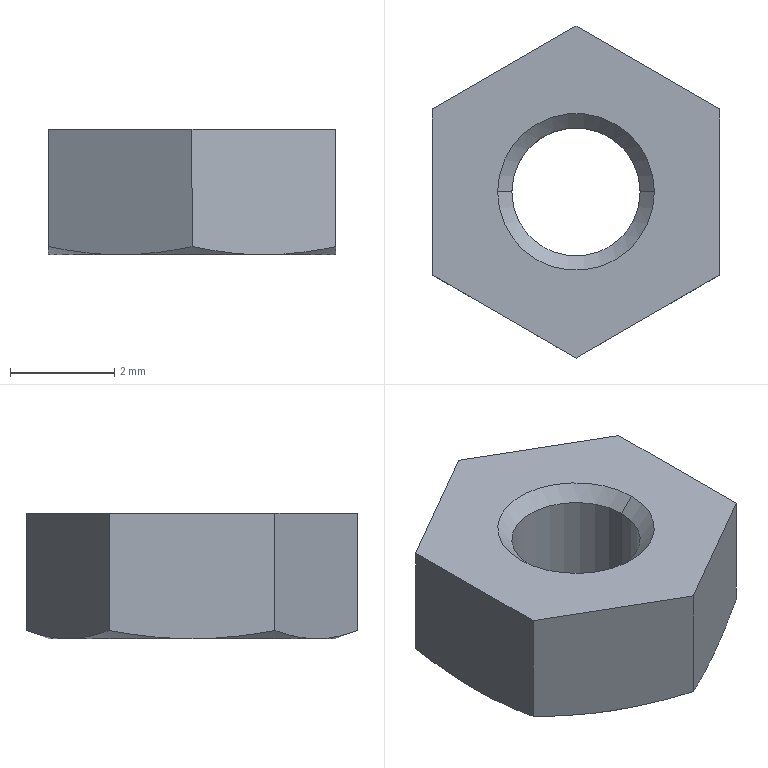Part | SolidWorks | features BaseBody 1 | 1 solid | 20 faces | box 5.5 x 6.351 x 2.4 mm | volume 50.752 mm3 | cone 10 | plane 8 | cylinder 2 | commonest cylinder face diameters 2.459 x2
STEP:
#1=CARTESIAN_POINT('',(-1.23,0.,2.13));
#2=VERTEX_POINT('',#1);
#3=CARTESIAN_POINT('',(1.23,0.,2.13));
#4=VERTEX_POINT('',#3);
#5=CARTESIAN_POINT('',(0.,0.,2.13));
#6=DIRECTION('',(0.,0.,1.));
#7=DIRECTION('',(1.,0.,0.));
#8=AXIS2_PLACEMENT_3D('',#5,#6,#7);
#9=CIRCLE('',#8,1.23);
#10=EDGE_CURVE('',#2,#4,#9,.T.);
#11=ORIENTED_EDGE('',*,*,#10,.F.);
#12=CARTESIAN_POINT('',(-1.5,0.,2.4));
#13=VERTEX_POINT('',#12);
#14=CARTESIAN_POINT('',(-1.5,0.,2.4));
#15=DIRECTION('',(-0.7071,0.,0.7071));
#16=VECTOR('',#15,1000.);
#17=LINE('',#14,#16);
#18=EDGE_CURVE('',#2,#13,#17,.T.);
#19=ORIENTED_EDGE('',*,*,#18,.T.);
#20=CARTESIAN_POINT('',(1.5,0.,2.4));
#21=VERTEX_POINT('',#20);
#22=CARTESIAN_POINT('',(0.,0.,2.4));
#23=DIRECTION('',(0.,0.,-1.));
#24=DIRECTION('',(1.,0.,0.));
#25=AXIS2_PLACEMENT_3D('',#22,#23,#24);
#26=CIRCLE('',#25,1.5);
#27=EDGE_CURVE('',#21,#13,#26,.T.);
#28=ORIENTED_EDGE('',*,*,#27,.F.);
#29=CARTESIAN_POINT('',(1.5,0.,2.4));
#30=DIRECTION('',(0.7071,0.,0.7071));
#31=VECTOR('',#30,1000.);
#32=LINE('',#29,#31);
#33=EDGE_CURVE('',#4,#21,#32,.T.);
#34=ORIENTED_EDGE('',*,*,#33,.F.);
#35=EDGE_LOOP('',(#11,#19,#28,#34));
#36=FACE_OUTER_BOUND('',#35,.T.);
#37=CARTESIAN_POINT('',(0.,0.,2.4));
#38=DIRECTION('',(0.,0.,1.));
#39=DIRECTION('',(1.,0.,0.));
#40=AXIS2_PLACEMENT_3D('',#37,#38,#39);
#41=CONICAL_SURFACE('',#40,1.5,0.7854);
#42=ADVANCED_FACE('',(#36),#41,.F.);
#43=CARTESIAN_POINT('',(-1.23,0.,0.2705));
#44=VERTEX_POINT('',#43);
#45=CARTESIAN_POINT('',(1.23,0.,0.2705));
#46=VERTEX_POINT('',#45);
#47=CARTESIAN_POINT('',(0.,0.,0.2705));
#48=DIRECTION('',(0.,0.,1.));
#49=DIRECTION('',(1.,0.,0.));
#50=AXIS2_PLACEMENT_3D('',#47,#48,#49);
#51=CIRCLE('',#50,1.23);
#52=EDGE_CURVE('',#44,#46,#51,.T.);
#53=ORIENTED_EDGE('',*,*,#52,.F.);
#54=CARTESIAN_POINT('',(-1.23,0.,0.));
#55=DIRECTION('',(0.,0.,1.));
#56=VECTOR('',#55,1000.);
#57=LINE('',#54,#56);
#58=EDGE_CURVE('',#44,#2,#57,.T.);
#59=ORIENTED_EDGE('',*,*,#58,.T.);
#60=ORIENTED_EDGE('',*,*,#10,.T.);
#61=CARTESIAN_POINT('',(1.23,0.,0.));
#62=DIRECTION('',(0.,0.,1.));
#63=VECTOR('',#62,1000.);
#64=LINE('',#61,#63);
#65=EDGE_CURVE('',#46,#4,#64,.T.);
#66=ORIENTED_EDGE('',*,*,#65,.F.);
#67=EDGE_LOOP('',(#53,#59,#60,#66));
#68=FACE_OUTER_BOUND('',#67,.T.);
#69=CARTESIAN_POINT('',(0.,0.,0.));
#70=DIRECTION('',(0.,0.,1.));
#71=DIRECTION('',(1.,0.,0.));
#72=AXIS2_PLACEMENT_3D('',#69,#70,#71);
#73=CYLINDRICAL_SURFACE('',#72,1.23);
#74=ADVANCED_FACE('',(#68),#73,.F.);
#75=ORIENTED_EDGE('',*,*,#52,.T.);
#76=CARTESIAN_POINT('',(1.5,0.,0.));
#77=VERTEX_POINT('',#76);
#78=CARTESIAN_POINT('',(1.5,0.,0.));
#79=DIRECTION('',(0.7071,0.,-0.7071));
#80=VECTOR('',#79,1000.);
#81=LINE('',#78,#80);
#82=EDGE_CURVE('',#46,#77,#81,.T.);
#83=ORIENTED_EDGE('',*,*,#82,.T.);
#84=CARTESIAN_POINT('',(-1.5,0.,0.));
#85=VERTEX_POINT('',#84);
#86=CARTESIAN_POINT('',(0.,0.,0.));
#87=DIRECTION('',(0.,0.,1.));
#88=DIRECTION('',(-1.,0.,0.));
#89=AXIS2_PLACEMENT_3D('',#86,#87,#88);
#90=CIRCLE('',#89,1.5);
#91=EDGE_CURVE('',#85,#77,#90,.T.);
#92=ORIENTED_EDGE('',*,*,#91,.F.);
#93=CARTESIAN_POINT('',(-1.5,0.,0.));
#94=DIRECTION('',(-0.7071,0.,-0.7071));
#95=VECTOR('',#94,1000.);
#96=LINE('',#93,#95);
#97=EDGE_CURVE('',#44,#85,#96,.T.);
#98=ORIENTED_EDGE('',*,*,#97,.F.);
#99=EDGE_LOOP('',(#75,#83,#92,#98));
#100=FACE_OUTER_BOUND('',#99,.T.);
#101=CARTESIAN_POINT('',(0.,0.,0.));
#102=DIRECTION('',(0.,0.,-1.));
#103=DIRECTION('',(-1.,0.,0.));
#104=AXIS2_PLACEMENT_3D('',#101,#102,#103);
#105=CONICAL_SURFACE('',#104,1.5,0.7854);
#106=ADVANCED_FACE('',(#100),#105,.F.);
#107=ORIENTED_EDGE('',*,*,#27,.T.);
#108=CARTESIAN_POINT('',(0.,0.,2.4));
#109=DIRECTION('',(0.,0.,-1.));
#110=DIRECTION('',(1.,0.,0.));
#111=AXIS2_PLACEMENT_3D('',#108,#109,#110);
#112=CIRCLE('',#111,1.5);
#113=EDGE_CURVE('',#13,#21,#112,.T.);
#114=ORIENTED_EDGE('',*,*,#113,.T.);
#115=EDGE_LOOP('',(#107,#114));
#116=FACE_BOUND('',#115,.T.);
#117=CARTESIAN_POINT('',(2.75,-1.588,2.4));
#118=VERTEX_POINT('',#117);
#119=CARTESIAN_POINT('',(2.75,1.588,2.4));
#120=VERTEX_POINT('',#119);
#121=CARTESIAN_POINT('',(2.75,0.,2.4));
#122=DIRECTION('',(0.,1.,0.));
#123=VECTOR('',#122,1000.);
#124=LINE('',#121,#123);
#125=EDGE_CURVE('',#118,#120,#124,.T.);
#126=ORIENTED_EDGE('',*,*,#125,.T.);
#127=CARTESIAN_POINT('',(0.,3.175,2.4));
#128=VERTEX_POINT('',#127);
#129=CARTESIAN_POINT('',(2.75,1.588,2.4));
#130=DIRECTION('',(-0.866,0.5,0.));
#131=VECTOR('',#130,1000.);
#132=LINE('',#129,#131);
#133=EDGE_CURVE('',#120,#128,#132,.T.);
#134=ORIENTED_EDGE('',*,*,#133,.T.);
#135=CARTESIAN_POINT('',(-2.75,1.588,2.4));
#136=VERTEX_POINT('',#135);
#137=CARTESIAN_POINT('',(0.,3.175,2.4));
#138=DIRECTION('',(-0.866,-0.5,0.));
#139=VECTOR('',#138,1000.);
#140=LINE('',#137,#139);
#141=EDGE_CURVE('',#128,#136,#140,.T.);
#142=ORIENTED_EDGE('',*,*,#141,.T.);
#143=CARTESIAN_POINT('',(-2.75,-1.588,2.4));
#144=VERTEX_POINT('',#143);
#145=CARTESIAN_POINT('',(-2.75,0.,2.4));
#146=DIRECTION('',(0.,-1.,0.));
#147=VECTOR('',#146,1000.);
#148=LINE('',#145,#147);
#149=EDGE_CURVE('',#136,#144,#148,.T.);
#150=ORIENTED_EDGE('',*,*,#149,.T.);
#151=CARTESIAN_POINT('',(0.,-3.175,2.4));
#152=VERTEX_POINT('',#151);
#153=CARTESIAN_POINT('',(-2.75,-1.588,2.4));
#154=DIRECTION('',(0.866,-0.5,0.));
#155=VECTOR('',#154,1000.);
#156=LINE('',#153,#155);
#157=EDGE_CURVE('',#144,#152,#156,.T.);
#158=ORIENTED_EDGE('',*,*,#157,.T.);
#159=CARTESIAN_POINT('',(0.,-3.175,2.4));
#160=DIRECTION('',(0.866,0.5,0.));
#161=VECTOR('',#160,1000.);
#162=LINE('',#159,#161);
#163=EDGE_CURVE('',#152,#118,#162,.T.);
#164=ORIENTED_EDGE('',*,*,#163,.T.);
#165=EDGE_LOOP('',(#126,#134,#142,#150,#158,#164));
#166=FACE_OUTER_BOUND('',#165,.T.);
#167=CARTESIAN_POINT('',(0.,0.,2.4));
#168=DIRECTION('',(0.,0.,1.));
#169=DIRECTION('',(1.,0.,0.));
#170=AXIS2_PLACEMENT_3D('',#167,#168,#169);
#171=PLANE('',#170);
#172=ADVANCED_FACE('',(#116,#166),#171,.T.);
#173=ORIENTED_EDGE('',*,*,#18,.F.);
#174=CARTESIAN_POINT('',(0.,0.,2.13));
#175=DIRECTION('',(0.,0.,1.));
#176=DIRECTION('',(1.,0.,0.));
#177=AXIS2_PLACEMENT_3D('',#174,#175,#176);
#178=CIRCLE('',#177,1.23);
#179=EDGE_CURVE('',#4,#2,#178,.T.);
#180=ORIENTED_EDGE('',*,*,#179,.F.);
#181=ORIENTED_EDGE('',*,*,#33,.T.);
#182=ORIENTED_EDGE('',*,*,#113,.F.);
#183=EDGE_LOOP('',(#173,#180,#181,#182));
#184=FACE_OUTER_BOUND('',#183,.T.);
#185=CARTESIAN_POINT('',(0.,0.,2.4));
#186=DIRECTION('',(0.,0.,1.));
#187=DIRECTION('',(1.,0.,0.));
#188=AXIS2_PLACEMENT_3D('',#185,#186,#187);
#189=CONICAL_SURFACE('',#188,1.5,0.7854);
#190=ADVANCED_FACE('',(#184),#189,.F.);
#191=CARTESIAN_POINT('',(1.375,2.382,0.));
#192=VERTEX_POINT('',#191);
#193=CARTESIAN_POINT('',(2.75,1.588,0.1548));
#194=VERTEX_POINT('',#193);
#195=CARTESIAN_POINT('',(1.375,2.382,0.));
#196=CARTESIAN_POINT('',(1.838,2.114,0.));
#197=CARTESIAN_POINT('',(2.295,1.85,0.05931));
#198=CARTESIAN_POINT('',(2.75,1.588,0.1548));
#199=B_SPLINE_CURVE_WITH_KNOTS('',3,(#195,#196,#197,#198),.UNSPECIFIED.,.F.,.F.,(4,4),(0.,0.001595),.UNSPECIFIED.);
#200=EDGE_CURVE('',#192,#194,#199,.T.);
#201=ORIENTED_EDGE('',*,*,#200,.F.);
#202=CARTESIAN_POINT('',(-0.000000018,3.175,0.1548));
#203=VERTEX_POINT('',#202);
#204=CARTESIAN_POINT('',(-0.000000018,3.175,0.1548));
#205=CARTESIAN_POINT('',(0.4546,2.913,0.05931));
#206=CARTESIAN_POINT('',(0.9123,2.649,0.));
#207=CARTESIAN_POINT('',(1.375,2.382,0.));
#208=B_SPLINE_CURVE_WITH_KNOTS('',3,(#204,#205,#206,#207),.UNSPECIFIED.,.F.,.F.,(4,4),(0.,0.001595),.UNSPECIFIED.);
#209=EDGE_CURVE('',#203,#192,#208,.T.);
#210=ORIENTED_EDGE('',*,*,#209,.F.);
#211=CARTESIAN_POINT('',(0.,3.175,2.4));
#212=DIRECTION('',(0.,0.,-1.));
#213=VECTOR('',#212,1000.);
#214=LINE('',#211,#213);
#215=EDGE_CURVE('',#128,#203,#214,.T.);
#216=ORIENTED_EDGE('',*,*,#215,.F.);
#217=ORIENTED_EDGE('',*,*,#133,.F.);
#218=CARTESIAN_POINT('',(2.75,1.588,2.4));
#219=DIRECTION('',(0.,0.,1.));
#220=VECTOR('',#219,1000.);
#221=LINE('',#218,#220);
#222=EDGE_CURVE('',#194,#120,#221,.T.);
#223=ORIENTED_EDGE('',*,*,#222,.F.);
#224=EDGE_LOOP('',(#201,#210,#216,#217,#223));
#225=FACE_OUTER_BOUND('',#224,.T.);
#226=CARTESIAN_POINT('',(2.75,1.588,2.4));
#227=DIRECTION('',(-0.5,-0.866,0.));
#228=DIRECTION('',(0.866,-0.5,0.));
#229=AXIS2_PLACEMENT_3D('',#226,#227,#228);
#230=PLANE('',#229);
#231=ADVANCED_FACE('',(#225),#230,.F.);
#232=CARTESIAN_POINT('',(2.75,0.,0.));
#233=VERTEX_POINT('',#232);
#234=CARTESIAN_POINT('',(2.75,-1.588,0.1548));
#235=VERTEX_POINT('',#234);
#236=CARTESIAN_POINT('',(2.75,0.,0.));
#237=CARTESIAN_POINT('',(2.75,-0.5343,0.));
#238=CARTESIAN_POINT('',(2.75,-1.063,0.05931));
#239=CARTESIAN_POINT('',(2.75,-1.588,0.1548));
#240=B_SPLINE_CURVE_WITH_KNOTS('',3,(#236,#237,#238,#239),.UNSPECIFIED.,.F.,.F.,(4,4),(0.,0.001595),.UNSPECIFIED.);
#241=EDGE_CURVE('',#233,#235,#240,.T.);
#242=ORIENTED_EDGE('',*,*,#241,.F.);
#243=CARTESIAN_POINT('',(2.75,1.588,0.1548));
#244=CARTESIAN_POINT('',(2.75,1.063,0.05931));
#245=CARTESIAN_POINT('',(2.75,0.5343,0.));
#246=CARTESIAN_POINT('',(2.75,0.,0.));
#247=B_SPLINE_CURVE_WITH_KNOTS('',3,(#243,#244,#245,#246),.UNSPECIFIED.,.F.,.F.,(4,4),(0.,0.001595),.UNSPECIFIED.);
#248=EDGE_CURVE('',#194,#233,#247,.T.);
#249=ORIENTED_EDGE('',*,*,#248,.F.);
#250=ORIENTED_EDGE('',*,*,#222,.T.);
#251=ORIENTED_EDGE('',*,*,#125,.F.);
#252=CARTESIAN_POINT('',(2.75,-1.588,2.4));
#253=DIRECTION('',(0.,0.,1.));
#254=VECTOR('',#253,1000.);
#255=LINE('',#252,#254);
#256=EDGE_CURVE('',#235,#118,#255,.T.);
#257=ORIENTED_EDGE('',*,*,#256,.F.);
#258=EDGE_LOOP('',(#242,#249,#250,#251,#257));
#259=FACE_OUTER_BOUND('',#258,.T.);
#260=CARTESIAN_POINT('',(2.75,-1.588,2.4));
#261=DIRECTION('',(-1.,0.,0.));
#262=DIRECTION('',(0.,0.,1.));
#263=AXIS2_PLACEMENT_3D('',#260,#261,#262);
#264=PLANE('',#263);
#265=ADVANCED_FACE('',(#259),#264,.F.);
#266=CARTESIAN_POINT('',(1.375,-2.382,0.));
#267=VERTEX_POINT('',#266);
#268=CARTESIAN_POINT('',(0.000000018,-3.175,0.1548));
#269=VERTEX_POINT('',#268);
#270=CARTESIAN_POINT('',(1.375,-2.382,0.));
#271=CARTESIAN_POINT('',(0.9123,-2.649,0.));
#272=CARTESIAN_POINT('',(0.4546,-2.913,0.05931));
#273=CARTESIAN_POINT('',(0.000000018,-3.175,0.1548));
#274=B_SPLINE_CURVE_WITH_KNOTS('',3,(#270,#271,#272,#273),.UNSPECIFIED.,.F.,.F.,(4,4),(0.,0.001595),.UNSPECIFIED.);
#275=EDGE_CURVE('',#267,#269,#274,.T.);
#276=ORIENTED_EDGE('',*,*,#275,.F.);
#277=CARTESIAN_POINT('',(2.75,-1.588,0.1548));
#278=CARTESIAN_POINT('',(2.295,-1.85,0.05931));
#279=CARTESIAN_POINT('',(1.838,-2.114,0.));
#280=CARTESIAN_POINT('',(1.375,-2.382,0.));
#281=B_SPLINE_CURVE_WITH_KNOTS('',3,(#277,#278,#279,#280),.UNSPECIFIED.,.F.,.F.,(4,4),(0.,0.001595),.UNSPECIFIED.);
#282=EDGE_CURVE('',#235,#267,#281,.T.);
#283=ORIENTED_EDGE('',*,*,#282,.F.);
#284=ORIENTED_EDGE('',*,*,#256,.T.);
#285=ORIENTED_EDGE('',*,*,#163,.F.);
#286=CARTESIAN_POINT('',(0.,-3.175,2.4));
#287=DIRECTION('',(0.,0.,1.));
#288=VECTOR('',#287,1000.);
#289=LINE('',#286,#288);
#290=EDGE_CURVE('',#269,#152,#289,.T.);
#291=ORIENTED_EDGE('',*,*,#290,.F.);
#292=EDGE_LOOP('',(#276,#283,#284,#285,#291));
#293=FACE_OUTER_BOUND('',#292,.T.);
#294=CARTESIAN_POINT('',(0.,-3.175,2.4));
#295=DIRECTION('',(-0.5,0.866,0.));
#296=DIRECTION('',(-0.866,-0.5,0.));
#297=AXIS2_PLACEMENT_3D('',#294,#295,#296);
#298=PLANE('',#297);
#299=ADVANCED_FACE('',(#293),#298,.F.);
#300=CARTESIAN_POINT('',(-1.375,-2.382,0.));
#301=VERTEX_POINT('',#300);
#302=CARTESIAN_POINT('',(-2.75,-1.588,0.1548));
#303=VERTEX_POINT('',#302);
#304=CARTESIAN_POINT('',(-1.375,-2.382,0.));
#305=CARTESIAN_POINT('',(-1.838,-2.114,0.));
#306=CARTESIAN_POINT('',(-2.295,-1.85,0.05931));
#307=CARTESIAN_POINT('',(-2.75,-1.588,0.1548));
#308=B_SPLINE_CURVE_WITH_KNOTS('',3,(#304,#305,#306,#307),.UNSPECIFIED.,.F.,.F.,(4,4),(0.,0.001595),.UNSPECIFIED.);
#309=EDGE_CURVE('',#301,#303,#308,.T.);
#310=ORIENTED_EDGE('',*,*,#309,.F.);
#311=CARTESIAN_POINT('',(0.000000018,-3.175,0.1548));
#312=CARTESIAN_POINT('',(-0.4546,-2.913,0.05931));
#313=CARTESIAN_POINT('',(-0.9123,-2.649,0.));
#314=CARTESIAN_POINT('',(-1.375,-2.382,0.));
#315=B_SPLINE_CURVE_WITH_KNOTS('',3,(#311,#312,#313,#314),.UNSPECIFIED.,.F.,.F.,(4,4),(0.,0.001595),.UNSPECIFIED.);
#316=EDGE_CURVE('',#269,#301,#315,.T.);
#317=ORIENTED_EDGE('',*,*,#316,.F.);
#318=ORIENTED_EDGE('',*,*,#290,.T.);
#319=ORIENTED_EDGE('',*,*,#157,.F.);
#320=CARTESIAN_POINT('',(-2.75,-1.588,2.4));
#321=DIRECTION('',(0.,0.,1.));
#322=VECTOR('',#321,1000.);
#323=LINE('',#320,#322);
#324=EDGE_CURVE('',#303,#144,#323,.T.);
#325=ORIENTED_EDGE('',*,*,#324,.F.);
#326=EDGE_LOOP('',(#310,#317,#318,#319,#325));
#327=FACE_OUTER_BOUND('',#326,.T.);
#328=CARTESIAN_POINT('',(-2.75,-1.588,2.4));
#329=DIRECTION('',(0.5,0.866,0.));
#330=DIRECTION('',(-0.866,0.5,0.));
#331=AXIS2_PLACEMENT_3D('',#328,#329,#330);
#332=PLANE('',#331);
#333=ADVANCED_FACE('',(#327),#332,.F.);
#334=CARTESIAN_POINT('',(-2.75,0.,0.));
#335=VERTEX_POINT('',#334);
#336=CARTESIAN_POINT('',(-2.75,1.588,0.1548));
#337=VERTEX_POINT('',#336);
#338=CARTESIAN_POINT('',(-2.75,0.,0.));
#339=CARTESIAN_POINT('',(-2.75,0.5343,0.));
#340=CARTESIAN_POINT('',(-2.75,1.063,0.05931));
#341=CARTESIAN_POINT('',(-2.75,1.588,0.1548));
#342=B_SPLINE_CURVE_WITH_KNOTS('',3,(#338,#339,#340,#341),.UNSPECIFIED.,.F.,.F.,(4,4),(0.,0.001595),.UNSPECIFIED.);
#343=EDGE_CURVE('',#335,#337,#342,.T.);
#344=ORIENTED_EDGE('',*,*,#343,.F.);
#345=CARTESIAN_POINT('',(-2.75,-1.588,0.1548));
#346=CARTESIAN_POINT('',(-2.75,-1.063,0.05931));
#347=CARTESIAN_POINT('',(-2.75,-0.5343,0.));
#348=CARTESIAN_POINT('',(-2.75,0.,0.));
#349=B_SPLINE_CURVE_WITH_KNOTS('',3,(#345,#346,#347,#348),.UNSPECIFIED.,.F.,.F.,(4,4),(0.,0.001595),.UNSPECIFIED.);
#350=EDGE_CURVE('',#303,#335,#349,.T.);
#351=ORIENTED_EDGE('',*,*,#350,.F.);
#352=ORIENTED_EDGE('',*,*,#324,.T.);
#353=ORIENTED_EDGE('',*,*,#149,.F.);
#354=CARTESIAN_POINT('',(-2.75,1.588,2.4));
#355=DIRECTION('',(0.,0.,1.));
#356=VECTOR('',#355,1000.);
#357=LINE('',#354,#356);
#358=EDGE_CURVE('',#337,#136,#357,.T.);
#359=ORIENTED_EDGE('',*,*,#358,.F.);
#360=EDGE_LOOP('',(#344,#351,#352,#353,#359));
#361=FACE_OUTER_BOUND('',#360,.T.);
#362=CARTESIAN_POINT('',(-2.75,1.588,2.4));
#363=DIRECTION('',(1.,0.,0.));
#364=DIRECTION('',(0.,0.,-1.));
#365=AXIS2_PLACEMENT_3D('',#362,#363,#364);
#366=PLANE('',#365);
#367=ADVANCED_FACE('',(#361),#366,.F.);
#368=CARTESIAN_POINT('',(-1.375,2.382,0.));
#369=VERTEX_POINT('',#368);
#370=CARTESIAN_POINT('',(-1.375,2.382,0.));
#371=CARTESIAN_POINT('',(-0.9123,2.649,0.));
#372=CARTESIAN_POINT('',(-0.4546,2.913,0.05931));
#373=CARTESIAN_POINT('',(-0.000000018,3.175,0.1548));
#374=B_SPLINE_CURVE_WITH_KNOTS('',3,(#370,#371,#372,#373),.UNSPECIFIED.,.F.,.F.,(4,4),(0.,0.001595),.UNSPECIFIED.);
#375=EDGE_CURVE('',#369,#203,#374,.T.);
#376=ORIENTED_EDGE('',*,*,#375,.F.);
#377=CARTESIAN_POINT('',(-2.75,1.588,0.1548));
#378=CARTESIAN_POINT('',(-2.295,1.85,0.05931));
#379=CARTESIAN_POINT('',(-1.838,2.114,0.));
#380=CARTESIAN_POINT('',(-1.375,2.382,0.));
#381=B_SPLINE_CURVE_WITH_KNOTS('',3,(#377,#378,#379,#380),.UNSPECIFIED.,.F.,.F.,(4,4),(0.,0.001595),.UNSPECIFIED.);
#382=EDGE_CURVE('',#337,#369,#381,.T.);
#383=ORIENTED_EDGE('',*,*,#382,.F.);
#384=ORIENTED_EDGE('',*,*,#358,.T.);
#385=ORIENTED_EDGE('',*,*,#141,.F.);
#386=ORIENTED_EDGE('',*,*,#215,.T.);
#387=EDGE_LOOP('',(#376,#383,#384,#385,#386));
#388=FACE_OUTER_BOUND('',#387,.T.);
#389=CARTESIAN_POINT('',(0.,3.175,2.4));
#390=DIRECTION('',(0.5,-0.866,0.));
#391=DIRECTION('',(0.866,0.5,0.));
#392=AXIS2_PLACEMENT_3D('',#389,#390,#391);
#393=PLANE('',#392);
#394=ADVANCED_FACE('',(#388),#393,.F.);
#395=ORIENTED_EDGE('',*,*,#58,.F.);
#396=CARTESIAN_POINT('',(0.,0.,0.2705));
#397=DIRECTION('',(0.,0.,1.));
#398=DIRECTION('',(1.,0.,0.));
#399=AXIS2_PLACEMENT_3D('',#396,#397,#398);
#400=CIRCLE('',#399,1.23);
#401=EDGE_CURVE('',#46,#44,#400,.T.);
#402=ORIENTED_EDGE('',*,*,#401,.F.);
#403=ORIENTED_EDGE('',*,*,#65,.T.);
#404=ORIENTED_EDGE('',*,*,#179,.T.);
#405=EDGE_LOOP('',(#395,#402,#403,#404));
#406=FACE_OUTER_BOUND('',#405,.T.);
#407=CARTESIAN_POINT('',(0.,0.,0.));
#408=DIRECTION('',(0.,0.,1.));
#409=DIRECTION('',(1.,0.,0.));
#410=AXIS2_PLACEMENT_3D('',#407,#408,#409);
#411=CYLINDRICAL_SURFACE('',#410,1.23);
#412=ADVANCED_FACE('',(#406),#411,.F.);
#413=ORIENTED_EDGE('',*,*,#343,.T.);
#414=ORIENTED_EDGE('',*,*,#382,.T.);
#415=CARTESIAN_POINT('',(0.,0.,0.));
#416=DIRECTION('',(0.,0.,1.));
#417=DIRECTION('',(1.,0.,0.));
#418=AXIS2_PLACEMENT_3D('',#415,#416,#417);
#419=CIRCLE('',#418,2.75);
#420=EDGE_CURVE('',#369,#335,#419,.T.);
#421=ORIENTED_EDGE('',*,*,#420,.T.);
#422=EDGE_LOOP('',(#413,#414,#421));
#423=FACE_OUTER_BOUND('',#422,.T.);
#424=CARTESIAN_POINT('',(0.,0.,0.1558));
#425=DIRECTION('',(0.,0.,1.));
#426=DIRECTION('',(1.,0.,0.));
#427=AXIS2_PLACEMENT_3D('',#424,#425,#426);
#428=CONICAL_SURFACE('',#427,3.178,1.222);
#429=ADVANCED_FACE('',(#423),#428,.T.);
#430=ORIENTED_EDGE('',*,*,#82,.F.);
#431=ORIENTED_EDGE('',*,*,#401,.T.);
#432=ORIENTED_EDGE('',*,*,#97,.T.);
#433=CARTESIAN_POINT('',(0.,0.,0.));
#434=DIRECTION('',(0.,0.,1.));
#435=DIRECTION('',(-1.,0.,0.));
#436=AXIS2_PLACEMENT_3D('',#433,#434,#435);
#437=CIRCLE('',#436,1.5);
#438=EDGE_CURVE('',#77,#85,#437,.T.);
#439=ORIENTED_EDGE('',*,*,#438,.F.);
#440=EDGE_LOOP('',(#430,#431,#432,#439));
#441=FACE_OUTER_BOUND('',#440,.T.);
#442=CARTESIAN_POINT('',(0.,0.,0.));
#443=DIRECTION('',(0.,0.,-1.));
#444=DIRECTION('',(-1.,0.,0.));
#445=AXIS2_PLACEMENT_3D('',#442,#443,#444);
#446=CONICAL_SURFACE('',#445,1.5,0.7854);
#447=ADVANCED_FACE('',(#441),#446,.F.);
#448=ORIENTED_EDGE('',*,*,#91,.T.);
#449=ORIENTED_EDGE('',*,*,#438,.T.);
#450=EDGE_LOOP('',(#448,#449));
#451=FACE_BOUND('',#450,.T.);
#452=CARTESIAN_POINT('',(0.,0.,0.));
#453=DIRECTION('',(0.,0.,1.));
#454=DIRECTION('',(1.,0.,0.));
#455=AXIS2_PLACEMENT_3D('',#452,#453,#454);
#456=CIRCLE('',#455,2.75);
#457=EDGE_CURVE('',#301,#267,#456,.T.);
#458=ORIENTED_EDGE('',*,*,#457,.F.);
#459=CARTESIAN_POINT('',(0.,0.,0.));
#460=DIRECTION('',(0.,0.,1.));
#461=DIRECTION('',(1.,0.,0.));
#462=AXIS2_PLACEMENT_3D('',#459,#460,#461);
#463=CIRCLE('',#462,2.75);
#464=EDGE_CURVE('',#335,#301,#463,.T.);
#465=ORIENTED_EDGE('',*,*,#464,.F.);
#466=ORIENTED_EDGE('',*,*,#420,.F.);
#467=CARTESIAN_POINT('',(0.,0.,0.));
#468=DIRECTION('',(0.,0.,1.));
#469=DIRECTION('',(1.,0.,0.));
#470=AXIS2_PLACEMENT_3D('',#467,#468,#469);
#471=CIRCLE('',#470,2.75);
#472=EDGE_CURVE('',#192,#369,#471,.T.);
#473=ORIENTED_EDGE('',*,*,#472,.F.);
#474=CARTESIAN_POINT('',(0.,0.,0.));
#475=DIRECTION('',(0.,0.,1.));
#476=DIRECTION('',(1.,0.,0.));
#477=AXIS2_PLACEMENT_3D('',#474,#475,#476);
#478=CIRCLE('',#477,2.75);
#479=EDGE_CURVE('',#233,#192,#478,.T.);
#480=ORIENTED_EDGE('',*,*,#479,.F.);
#481=CARTESIAN_POINT('',(0.,0.,0.));
#482=DIRECTION('',(0.,0.,1.));
#483=DIRECTION('',(1.,0.,0.));
#484=AXIS2_PLACEMENT_3D('',#481,#482,#483);
#485=CIRCLE('',#484,2.75);
#486=EDGE_CURVE('',#267,#233,#485,.T.);
#487=ORIENTED_EDGE('',*,*,#486,.F.);
#488=EDGE_LOOP('',(#458,#465,#466,#473,#480,#487));
#489=FACE_OUTER_BOUND('',#488,.T.);
#490=CARTESIAN_POINT('',(0.,0.,0.));
#491=DIRECTION('',(0.,0.,1.));
#492=DIRECTION('',(1.,0.,0.));
#493=AXIS2_PLACEMENT_3D('',#490,#491,#492);
#494=PLANE('',#493);
#495=ADVANCED_FACE('',(#451,#489),#494,.F.);
#496=ORIENTED_EDGE('',*,*,#241,.T.);
#497=ORIENTED_EDGE('',*,*,#282,.T.);
#498=ORIENTED_EDGE('',*,*,#486,.T.);
#499=EDGE_LOOP('',(#496,#497,#498));
#500=FACE_OUTER_BOUND('',#499,.T.);
#501=CARTESIAN_POINT('',(0.,0.,0.1558));
#502=DIRECTION('',(0.,0.,1.));
#503=DIRECTION('',(1.,0.,0.));
#504=AXIS2_PLACEMENT_3D('',#501,#502,#503);
#505=CONICAL_SURFACE('',#504,3.178,1.222);
#506=ADVANCED_FACE('',(#500),#505,.T.);
#507=ORIENTED_EDGE('',*,*,#275,.T.);
#508=ORIENTED_EDGE('',*,*,#316,.T.);
#509=ORIENTED_EDGE('',*,*,#457,.T.);
#510=EDGE_LOOP('',(#507,#508,#509));
#511=FACE_OUTER_BOUND('',#510,.T.);
#512=CARTESIAN_POINT('',(0.,0.,0.1558));
#513=DIRECTION('',(0.,0.,1.));
#514=DIRECTION('',(1.,0.,0.));
#515=AXIS2_PLACEMENT_3D('',#512,#513,#514);
#516=CONICAL_SURFACE('',#515,3.178,1.222);
#517=ADVANCED_FACE('',(#511),#516,.T.);
#518=ORIENTED_EDGE('',*,*,#309,.T.);
#519=ORIENTED_EDGE('',*,*,#350,.T.);
#520=ORIENTED_EDGE('',*,*,#464,.T.);
#521=EDGE_LOOP('',(#518,#519,#520));
#522=FACE_OUTER_BOUND('',#521,.T.);
#523=CARTESIAN_POINT('',(0.,0.,0.1558));
#524=DIRECTION('',(0.,0.,1.));
#525=DIRECTION('',(1.,0.,0.));
#526=AXIS2_PLACEMENT_3D('',#523,#524,#525);
#527=CONICAL_SURFACE('',#526,3.178,1.222);
#528=ADVANCED_FACE('',(#522),#527,.T.);
#529=ORIENTED_EDGE('',*,*,#209,.T.);
#530=ORIENTED_EDGE('',*,*,#472,.T.);
#531=ORIENTED_EDGE('',*,*,#375,.T.);
#532=EDGE_LOOP('',(#529,#530,#531));
#533=FACE_OUTER_BOUND('',#532,.T.);
#534=CARTESIAN_POINT('',(0.,0.,0.1558));
#535=DIRECTION('',(0.,0.,1.));
#536=DIRECTION('',(1.,0.,0.));
#537=AXIS2_PLACEMENT_3D('',#534,#535,#536);
#538=CONICAL_SURFACE('',#537,3.178,1.222);
#539=ADVANCED_FACE('',(#533),#538,.T.);
#540=ORIENTED_EDGE('',*,*,#200,.T.);
#541=ORIENTED_EDGE('',*,*,#248,.T.);
#542=ORIENTED_EDGE('',*,*,#479,.T.);
#543=EDGE_LOOP('',(#540,#541,#542));
#544=FACE_OUTER_BOUND('',#543,.T.);
#545=CARTESIAN_POINT('',(0.,0.,0.1558));
#546=DIRECTION('',(0.,0.,1.));
#547=DIRECTION('',(1.,0.,0.));
#548=AXIS2_PLACEMENT_3D('',#545,#546,#547);
#549=CONICAL_SURFACE('',#548,3.178,1.222);
#550=ADVANCED_FACE('',(#544),#549,.T.);
#551=CLOSED_SHELL('',(#42,#74,#106,#172,#190,#231,#265,#299,#333,#367,#394,#412,#429,#447,#495,#506,#517,#528,#539,#550));
#552=MANIFOLD_SOLID_BREP('',#551);
#553=CARTESIAN_POINT('',(0.,0.,0.));
#554=DIRECTION('',(0.,0.,1.));
#555=DIRECTION('',(1.,0.,0.));
#556=AXIS2_PLACEMENT_3D('',#553,#554,#555);
#557=(LENGTH_UNIT()NAMED_UNIT(*)SI_UNIT(.MILLI.,.METRE.));
#558=UNCERTAINTY_MEASURE_WITH_UNIT(LENGTH_MEASURE(0.00001),#557,'','');
#559=(NAMED_UNIT(*)PLANE_ANGLE_UNIT()SI_UNIT($,.RADIAN.));
#560=(NAMED_UNIT(*)SI_UNIT($,.STERADIAN.)SOLID_ANGLE_UNIT());
#561=(GEOMETRIC_REPRESENTATION_CONTEXT(3)GLOBAL_UNCERTAINTY_ASSIGNED_CONTEXT((#558))GLOBAL_UNIT_ASSIGNED_CONTEXT((#557,#559,#560))REPRESENTATION_CONTEXT('',''));
#562=ADVANCED_BREP_SHAPE_REPRESENTATION('',(#552,#556),#561);